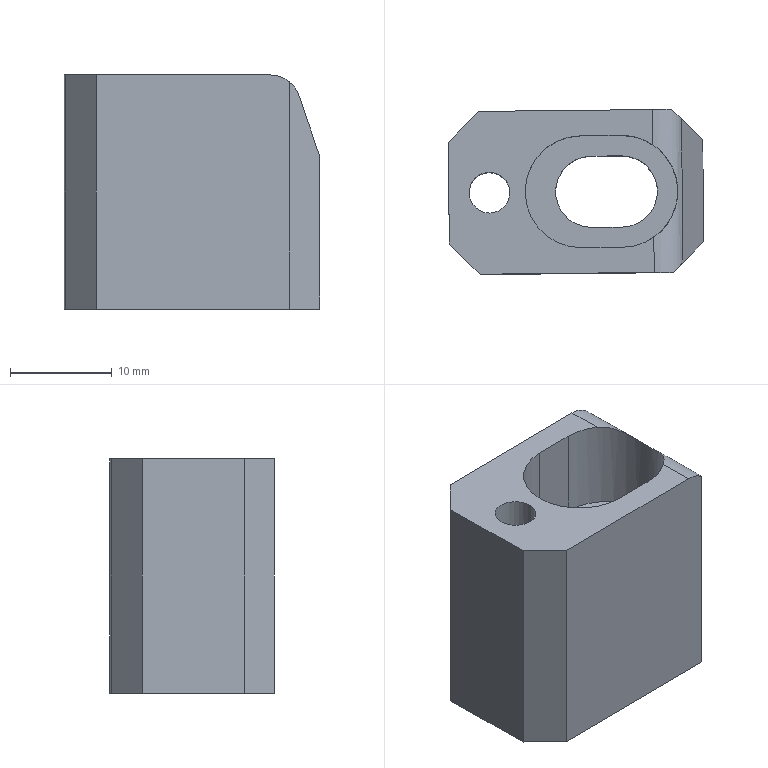Part | NX | features solid 2 | 1 solid | 22 faces | box 25.103 x 16.198 x 23 mm | volume 6273 mm3 | plane 16 | cylinder 6 | commonest cylinder face diameters 7 x2 11 x2 4.001 x1 6 x1
STEP:
#1=CARTESIAN_POINT('',(1618.85,-304.866,17.4));
#2=VERTEX_POINT('',#1);
#3=CARTESIAN_POINT('',(1635.95,-304.687,17.4));
#4=VERTEX_POINT('',#3);
#5=CARTESIAN_POINT('',(1630.849,-304.74,17.4));
#6=DIRECTION('',(0.9999,0.01047,0.));
#7=VECTOR('',#6,1000.);
#8=LINE('',#5,#7);
#9=EDGE_CURVE('',#2,#4,#8,.T.);
#10=ORIENTED_EDGE('',*,*,#9,.F.);
#11=CARTESIAN_POINT('',(1615.881,-307.897,17.4));
#12=VERTEX_POINT('',#11);
#13=CARTESIAN_POINT('',(1620.334,-303.35,17.4));
#14=DIRECTION('',(-0.6997,-0.7145,0.));
#15=VECTOR('',#14,1000.);
#16=LINE('',#13,#15);
#17=EDGE_CURVE('',#2,#12,#16,.T.);
#18=ORIENTED_EDGE('',*,*,#17,.T.);
#19=CARTESIAN_POINT('',(1615.986,-317.896,17.4));
#20=VERTEX_POINT('',#19);
#21=CARTESIAN_POINT('',(1615.934,-312.897,17.4));
#22=DIRECTION('',(-0.01047,0.9999,0.));
#23=VECTOR('',#22,1000.);
#24=LINE('',#21,#23);
#25=EDGE_CURVE('',#20,#12,#24,.T.);
#26=ORIENTED_EDGE('',*,*,#25,.F.);
#27=CARTESIAN_POINT('',(1619.017,-320.865,17.4));
#28=VERTEX_POINT('',#27);
#29=CARTESIAN_POINT('',(1620.533,-322.349,17.4));
#30=DIRECTION('',(0.7145,-0.6997,0.));
#31=VECTOR('',#30,1000.);
#32=LINE('',#29,#31);
#33=EDGE_CURVE('',#20,#28,#32,.T.);
#34=ORIENTED_EDGE('',*,*,#33,.T.);
#35=CARTESIAN_POINT('',(1636.118,-320.686,17.4));
#36=VERTEX_POINT('',#35);
#37=CARTESIAN_POINT('',(1631.017,-320.739,17.4));
#38=DIRECTION('',(-0.9999,-0.01047,0.));
#39=VECTOR('',#38,1000.);
#40=LINE('',#37,#39);
#41=EDGE_CURVE('',#36,#28,#40,.T.);
#42=ORIENTED_EDGE('',*,*,#41,.F.);
#43=CARTESIAN_POINT('',(1636.081,-317.228,17.4));
#44=VERTEX_POINT('',#43);
#45=CARTESIAN_POINT('',(1636.034,-312.686,17.4));
#46=DIRECTION('',(-0.01047,0.9999,0.));
#47=VECTOR('',#46,1000.);
#48=LINE('',#45,#47);
#49=EDGE_CURVE('',#36,#44,#48,.T.);
#50=ORIENTED_EDGE('',*,*,#49,.T.);
#51=CARTESIAN_POINT('',(1632.99,-318.218,17.4));
#52=VERTEX_POINT('',#51);
#53=CARTESIAN_POINT('',(1632.933,-312.719,17.4));
#54=DIRECTION('',(0.,0.,-1.));
#55=DIRECTION('',(-0.1736,0.9848,0.));
#56=AXIS2_PLACEMENT_3D('',#53,#54,#55);
#57=CIRCLE('',#56,5.5);
#58=EDGE_CURVE('',#44,#52,#57,.T.);
#59=ORIENTED_EDGE('',*,*,#58,.T.);
#60=CARTESIAN_POINT('',(1628.99,-318.26,17.4));
#61=VERTEX_POINT('',#60);
#62=CARTESIAN_POINT('',(1630.99,-318.239,17.4));
#63=DIRECTION('',(-0.9999,-0.01047,0.));
#64=VECTOR('',#63,1000.);
#65=LINE('',#62,#64);
#66=EDGE_CURVE('',#52,#61,#65,.T.);
#67=ORIENTED_EDGE('',*,*,#66,.T.);
#68=CARTESIAN_POINT('',(1628.875,-307.261,17.4));
#69=VERTEX_POINT('',#68);
#70=CARTESIAN_POINT('',(1628.933,-312.761,17.4));
#71=DIRECTION('',(0.,0.,-1.));
#72=DIRECTION('',(-0.1736,0.9848,0.));
#73=AXIS2_PLACEMENT_3D('',#70,#71,#72);
#74=CIRCLE('',#73,5.5);
#75=EDGE_CURVE('',#61,#69,#74,.T.);
#76=ORIENTED_EDGE('',*,*,#75,.T.);
#77=CARTESIAN_POINT('',(1632.875,-307.219,17.4));
#78=VERTEX_POINT('',#77);
#79=CARTESIAN_POINT('',(1630.875,-307.24,17.4));
#80=DIRECTION('',(0.9999,0.01047,0.));
#81=VECTOR('',#80,1000.);
#82=LINE('',#79,#81);
#83=EDGE_CURVE('',#69,#78,#82,.T.);
#84=ORIENTED_EDGE('',*,*,#83,.T.);
#85=CARTESIAN_POINT('',(1635.986,-308.144,17.4));
#86=VERTEX_POINT('',#85);
#87=CARTESIAN_POINT('',(1632.933,-312.719,17.4));
#88=DIRECTION('',(0.,0.,-1.));
#89=DIRECTION('',(-0.1736,0.9848,0.));
#90=AXIS2_PLACEMENT_3D('',#87,#88,#89);
#91=CIRCLE('',#90,5.5);
#92=EDGE_CURVE('',#78,#86,#91,.T.);
#93=ORIENTED_EDGE('',*,*,#92,.T.);
#94=CARTESIAN_POINT('',(1636.034,-312.686,17.4));
#95=DIRECTION('',(-0.01047,0.9999,0.));
#96=VECTOR('',#95,1000.);
#97=LINE('',#94,#96);
#98=EDGE_CURVE('',#86,#4,#97,.T.);
#99=ORIENTED_EDGE('',*,*,#98,.T.);
#100=EDGE_LOOP('',(#10,#18,#26,#34,#42,#50,#59,#67,#76,#84,#93,#99));
#101=FACE_BOUND('',#100,.T.);
#102=CARTESIAN_POINT('',(1619.49,-314.806,17.4));
#103=VERTEX_POINT('',#102);
#104=CARTESIAN_POINT('',(1619.933,-312.855,17.4));
#105=DIRECTION('',(0.,0.,-1.));
#106=DIRECTION('',(-0.2215,-0.9751,0.));
#107=AXIS2_PLACEMENT_3D('',#104,#105,#106);
#108=CIRCLE('',#107,2.001);
#109=EDGE_CURVE('',#103,#103,#108,.T.);
#110=ORIENTED_EDGE('',*,*,#109,.T.);
#111=EDGE_LOOP('',(#110));
#112=FACE_BOUND('',#111,.T.);
#113=CARTESIAN_POINT('',(1630.933,-312.74,17.4));
#114=DIRECTION('',(0.,0.,1.));
#115=DIRECTION('',(0.184,-0.9829,0.));
#116=AXIS2_PLACEMENT_3D('',#113,#114,#115);
#117=PLANE('',#116);
#118=ADVANCED_FACE('',(#101,#112),#117,.T.);
#119=CARTESIAN_POINT('',(1620.417,-314.796,-5.6));
#120=VERTEX_POINT('',#119);
#121=CARTESIAN_POINT('',(1619.933,-312.855,-5.6));
#122=DIRECTION('',(0.,0.,-1.));
#123=DIRECTION('',(0.2419,-0.9703,0.));
#124=AXIS2_PLACEMENT_3D('',#121,#122,#123);
#125=CIRCLE('',#124,2.001);
#126=EDGE_CURVE('',#120,#120,#125,.T.);
#127=ORIENTED_EDGE('',*,*,#126,.F.);
#128=EDGE_LOOP('',(#127));
#129=FACE_BOUND('',#128,.T.);
#130=CARTESIAN_POINT('',(1637.849,-304.667,-5.6));
#131=VERTEX_POINT('',#130);
#132=CARTESIAN_POINT('',(1618.85,-304.866,-5.6));
#133=VERTEX_POINT('',#132);
#134=CARTESIAN_POINT('',(1630.849,-304.74,-5.6));
#135=DIRECTION('',(-0.9999,-0.01047,0.));
#136=VECTOR('',#135,1000.);
#137=LINE('',#134,#136);
#138=EDGE_CURVE('',#131,#133,#137,.T.);
#139=ORIENTED_EDGE('',*,*,#138,.F.);
#140=CARTESIAN_POINT('',(1640.88,-307.635,-5.6));
#141=VERTEX_POINT('',#140);
#142=CARTESIAN_POINT('',(1638.354,-305.161,-5.6));
#143=DIRECTION('',(0.7145,-0.6997,0.));
#144=VECTOR('',#143,1000.);
#145=LINE('',#142,#144);
#146=EDGE_CURVE('',#131,#141,#145,.T.);
#147=ORIENTED_EDGE('',*,*,#146,.T.);
#148=CARTESIAN_POINT('',(1640.985,-317.635,-5.6));
#149=VERTEX_POINT('',#148);
#150=CARTESIAN_POINT('',(1640.932,-312.635,-5.6));
#151=DIRECTION('',(-0.01047,0.9999,0.));
#152=VECTOR('',#151,1000.);
#153=LINE('',#150,#152);
#154=EDGE_CURVE('',#149,#141,#153,.T.);
#155=ORIENTED_EDGE('',*,*,#154,.F.);
#156=CARTESIAN_POINT('',(1638.016,-320.666,-5.6));
#157=VERTEX_POINT('',#156);
#158=CARTESIAN_POINT('',(1638.511,-320.161,-5.6));
#159=DIRECTION('',(-0.6997,-0.7145,0.));
#160=VECTOR('',#159,1000.);
#161=LINE('',#158,#160);
#162=EDGE_CURVE('',#149,#157,#161,.T.);
#163=ORIENTED_EDGE('',*,*,#162,.T.);
#164=CARTESIAN_POINT('',(1619.017,-320.865,-5.6));
#165=VERTEX_POINT('',#164);
#166=CARTESIAN_POINT('',(1631.017,-320.739,-5.6));
#167=DIRECTION('',(0.9999,0.01047,0.));
#168=VECTOR('',#167,1000.);
#169=LINE('',#166,#168);
#170=EDGE_CURVE('',#165,#157,#169,.T.);
#171=ORIENTED_EDGE('',*,*,#170,.F.);
#172=CARTESIAN_POINT('',(1615.986,-317.896,-5.6));
#173=VERTEX_POINT('',#172);
#174=CARTESIAN_POINT('',(1620.028,-321.854,-5.6));
#175=DIRECTION('',(-0.7145,0.6997,0.));
#176=VECTOR('',#175,1000.);
#177=LINE('',#174,#176);
#178=EDGE_CURVE('',#165,#173,#177,.T.);
#179=ORIENTED_EDGE('',*,*,#178,.T.);
#180=CARTESIAN_POINT('',(1615.881,-307.897,-5.6));
#181=VERTEX_POINT('',#180);
#182=CARTESIAN_POINT('',(1615.934,-312.897,-5.6));
#183=DIRECTION('',(0.01047,-0.9999,0.));
#184=VECTOR('',#183,1000.);
#185=LINE('',#182,#184);
#186=EDGE_CURVE('',#181,#173,#185,.T.);
#187=ORIENTED_EDGE('',*,*,#186,.F.);
#188=CARTESIAN_POINT('',(1619.839,-303.855,-5.6));
#189=DIRECTION('',(0.6997,0.7145,0.));
#190=VECTOR('',#189,1000.);
#191=LINE('',#188,#190);
#192=EDGE_CURVE('',#181,#133,#191,.T.);
#193=ORIENTED_EDGE('',*,*,#192,.T.);
#194=EDGE_LOOP('',(#139,#147,#155,#163,#171,#179,#187,#193));
#195=FACE_BOUND('',#194,.T.);
#196=CARTESIAN_POINT('',(1632.969,-316.218,-5.6));
#197=VERTEX_POINT('',#196);
#198=CARTESIAN_POINT('',(1632.896,-309.219,-5.6));
#199=VERTEX_POINT('',#198);
#200=CARTESIAN_POINT('',(1632.933,-312.719,-5.6));
#201=DIRECTION('',(0.,0.,1.));
#202=DIRECTION('',(0.2419,-0.9703,0.));
#203=AXIS2_PLACEMENT_3D('',#200,#201,#202);
#204=CIRCLE('',#203,3.5);
#205=EDGE_CURVE('',#197,#199,#204,.T.);
#206=ORIENTED_EDGE('',*,*,#205,.T.);
#207=CARTESIAN_POINT('',(1629.896,-309.25,-5.6));
#208=VERTEX_POINT('',#207);
#209=CARTESIAN_POINT('',(1630.896,-309.24,-5.6));
#210=DIRECTION('',(-0.9999,-0.01047,0.));
#211=VECTOR('',#210,1000.);
#212=LINE('',#209,#211);
#213=EDGE_CURVE('',#199,#208,#212,.T.);
#214=ORIENTED_EDGE('',*,*,#213,.T.);
#215=CARTESIAN_POINT('',(1629.969,-316.25,-5.6));
#216=VERTEX_POINT('',#215);
#217=CARTESIAN_POINT('',(1629.933,-312.75,-5.6));
#218=DIRECTION('',(0.,0.,1.));
#219=DIRECTION('',(0.2419,-0.9703,0.));
#220=AXIS2_PLACEMENT_3D('',#217,#218,#219);
#221=CIRCLE('',#220,3.5);
#222=EDGE_CURVE('',#208,#216,#221,.T.);
#223=ORIENTED_EDGE('',*,*,#222,.T.);
#224=CARTESIAN_POINT('',(1630.969,-316.239,-5.6));
#225=DIRECTION('',(0.9999,0.01047,0.));
#226=VECTOR('',#225,1000.);
#227=LINE('',#224,#226);
#228=EDGE_CURVE('',#216,#197,#227,.T.);
#229=ORIENTED_EDGE('',*,*,#228,.T.);
#230=EDGE_LOOP('',(#206,#214,#223,#229));
#231=FACE_BOUND('',#230,.T.);
#232=CARTESIAN_POINT('',(1630.933,-312.74,-5.6));
#233=DIRECTION('',(0.,0.,-1.));
#234=DIRECTION('',(-0.184,0.9829,0.));
#235=AXIS2_PLACEMENT_3D('',#232,#233,#234);
#236=PLANE('',#235);
#237=ADVANCED_FACE('',(#129,#195,#231),#236,.T.);
#238=ORIENTED_EDGE('',*,*,#154,.T.);
#239=CARTESIAN_POINT('',(1640.88,-307.635,9.4));
#240=VERTEX_POINT('',#239);
#241=CARTESIAN_POINT('',(1640.88,-307.635,2.4));
#242=DIRECTION('',(0.,0.,1.));
#243=VECTOR('',#242,1000.);
#244=LINE('',#241,#243);
#245=EDGE_CURVE('',#141,#240,#244,.T.);
#246=ORIENTED_EDGE('',*,*,#245,.T.);
#247=CARTESIAN_POINT('',(1640.985,-317.635,9.4));
#248=VERTEX_POINT('',#247);
#249=CARTESIAN_POINT('',(1640.932,-312.635,9.4));
#250=DIRECTION('',(0.01047,-0.9999,0.));
#251=VECTOR('',#250,1000.);
#252=LINE('',#249,#251);
#253=EDGE_CURVE('',#240,#248,#252,.T.);
#254=ORIENTED_EDGE('',*,*,#253,.T.);
#255=CARTESIAN_POINT('',(1640.985,-317.635,2.4));
#256=DIRECTION('',(0.,0.,-1.));
#257=VECTOR('',#256,1000.);
#258=LINE('',#255,#257);
#259=EDGE_CURVE('',#248,#149,#258,.T.);
#260=ORIENTED_EDGE('',*,*,#259,.T.);
#261=EDGE_LOOP('',(#238,#246,#254,#260));
#262=FACE_BOUND('',#261,.T.);
#263=CARTESIAN_POINT('',(1640.932,-312.635,2.4));
#264=DIRECTION('',(0.9999,0.01047,0.));
#265=DIRECTION('',(0.01047,-0.9999,0.));
#266=AXIS2_PLACEMENT_3D('',#263,#264,#265);
#267=PLANE('',#266);
#268=ADVANCED_FACE('',(#262),#267,.T.);
#269=ORIENTED_EDGE('',*,*,#170,.T.);
#270=CARTESIAN_POINT('',(1638.016,-320.666,16.723));
#271=VERTEX_POINT('',#270);
#272=CARTESIAN_POINT('',(1638.016,-320.666,2.4));
#273=DIRECTION('',(0.,0.,1.));
#274=VECTOR('',#273,1000.);
#275=LINE('',#272,#274);
#276=EDGE_CURVE('',#157,#271,#275,.T.);
#277=ORIENTED_EDGE('',*,*,#276,.T.);
#278=CARTESIAN_POINT('',(1636.118,-320.686,14.4));
#279=DIRECTION('',(0.01047,-0.9999,0.));
#280=DIRECTION('',(0.9999,0.01047,0.));
#281=AXIS2_PLACEMENT_3D('',#278,#279,#280);
#282=CIRCLE('',#281,3.);
#283=EDGE_CURVE('',#271,#36,#282,.T.);
#284=ORIENTED_EDGE('',*,*,#283,.T.);
#285=ORIENTED_EDGE('',*,*,#41,.T.);
#286=CARTESIAN_POINT('',(1619.017,-320.865,2.4));
#287=DIRECTION('',(0.,0.,-1.));
#288=VECTOR('',#287,1000.);
#289=LINE('',#286,#288);
#290=EDGE_CURVE('',#28,#165,#289,.T.);
#291=ORIENTED_EDGE('',*,*,#290,.T.);
#292=EDGE_LOOP('',(#269,#277,#284,#285,#291));
#293=FACE_BOUND('',#292,.T.);
#294=CARTESIAN_POINT('',(1631.017,-320.739,2.4));
#295=DIRECTION('',(0.01047,-0.9999,0.));
#296=DIRECTION('',(-0.9999,-0.01047,0.));
#297=AXIS2_PLACEMENT_3D('',#294,#295,#296);
#298=PLANE('',#297);
#299=ADVANCED_FACE('',(#293),#298,.T.);
#300=ORIENTED_EDGE('',*,*,#25,.T.);
#301=CARTESIAN_POINT('',(1615.881,-307.897,2.4));
#302=DIRECTION('',(0.,0.,-1.));
#303=VECTOR('',#302,1000.);
#304=LINE('',#301,#303);
#305=EDGE_CURVE('',#12,#181,#304,.T.);
#306=ORIENTED_EDGE('',*,*,#305,.T.);
#307=ORIENTED_EDGE('',*,*,#186,.T.);
#308=CARTESIAN_POINT('',(1615.986,-317.896,2.4));
#309=DIRECTION('',(0.,0.,1.));
#310=VECTOR('',#309,1000.);
#311=LINE('',#308,#310);
#312=EDGE_CURVE('',#173,#20,#311,.T.);
#313=ORIENTED_EDGE('',*,*,#312,.T.);
#314=EDGE_LOOP('',(#300,#306,#307,#313));
#315=FACE_BOUND('',#314,.T.);
#316=CARTESIAN_POINT('',(1615.934,-312.897,2.4));
#317=DIRECTION('',(-0.9999,-0.01047,0.));
#318=DIRECTION('',(-0.01047,0.9999,0.));
#319=AXIS2_PLACEMENT_3D('',#316,#317,#318);
#320=PLANE('',#319);
#321=ADVANCED_FACE('',(#315),#320,.T.);
#322=CARTESIAN_POINT('',(1637.849,-304.667,16.723));
#323=VERTEX_POINT('',#322);
#324=CARTESIAN_POINT('',(1635.95,-304.687,14.4));
#325=DIRECTION('',(-0.01047,0.9999,0.));
#326=DIRECTION('',(-0.9999,-0.01047,0.));
#327=AXIS2_PLACEMENT_3D('',#324,#325,#326);
#328=CIRCLE('',#327,3.);
#329=EDGE_CURVE('',#4,#323,#328,.T.);
#330=ORIENTED_EDGE('',*,*,#329,.T.);
#331=CARTESIAN_POINT('',(1637.849,-304.667,2.4));
#332=DIRECTION('',(0.,0.,-1.));
#333=VECTOR('',#332,1000.);
#334=LINE('',#331,#333);
#335=EDGE_CURVE('',#323,#131,#334,.T.);
#336=ORIENTED_EDGE('',*,*,#335,.T.);
#337=ORIENTED_EDGE('',*,*,#138,.T.);
#338=CARTESIAN_POINT('',(1618.85,-304.866,2.4));
#339=DIRECTION('',(0.,0.,1.));
#340=VECTOR('',#339,1000.);
#341=LINE('',#338,#340);
#342=EDGE_CURVE('',#133,#2,#341,.T.);
#343=ORIENTED_EDGE('',*,*,#342,.T.);
#344=ORIENTED_EDGE('',*,*,#9,.T.);
#345=EDGE_LOOP('',(#330,#336,#337,#343,#344));
#346=FACE_BOUND('',#345,.T.);
#347=CARTESIAN_POINT('',(1630.849,-304.74,2.4));
#348=DIRECTION('',(-0.01047,0.9999,0.));
#349=DIRECTION('',(0.9999,0.01047,0.));
#350=AXIS2_PLACEMENT_3D('',#347,#348,#349);
#351=PLANE('',#350);
#352=ADVANCED_FACE('',(#346),#351,.T.);
#353=CARTESIAN_POINT('',(1629.896,-309.25,8.4));
#354=VERTEX_POINT('',#353);
#355=CARTESIAN_POINT('',(1629.969,-316.25,8.4));
#356=VERTEX_POINT('',#355);
#357=CARTESIAN_POINT('',(1629.933,-312.75,8.4));
#358=DIRECTION('',(0.,0.,1.));
#359=DIRECTION('',(0.1736,-0.9848,0.));
#360=AXIS2_PLACEMENT_3D('',#357,#358,#359);
#361=CIRCLE('',#360,3.5);
#362=EDGE_CURVE('',#354,#356,#361,.T.);
#363=ORIENTED_EDGE('',*,*,#362,.F.);
#364=CARTESIAN_POINT('',(1632.896,-309.219,8.4));
#365=VERTEX_POINT('',#364);
#366=CARTESIAN_POINT('',(1629.995,-309.249,8.4));
#367=DIRECTION('',(0.9999,0.01047,0.));
#368=VECTOR('',#367,1000.);
#369=LINE('',#366,#368);
#370=EDGE_CURVE('',#354,#365,#369,.T.);
#371=ORIENTED_EDGE('',*,*,#370,.T.);
#372=CARTESIAN_POINT('',(1632.969,-316.218,8.4));
#373=VERTEX_POINT('',#372);
#374=CARTESIAN_POINT('',(1632.933,-312.719,8.4));
#375=DIRECTION('',(0.,0.,-1.));
#376=DIRECTION('',(0.1736,-0.9848,0.));
#377=AXIS2_PLACEMENT_3D('',#374,#375,#376);
#378=CIRCLE('',#377,3.5);
#379=EDGE_CURVE('',#365,#373,#378,.T.);
#380=ORIENTED_EDGE('',*,*,#379,.T.);
#381=CARTESIAN_POINT('',(1630.068,-316.249,8.4));
#382=DIRECTION('',(-0.9999,-0.01047,0.));
#383=VECTOR('',#382,1000.);
#384=LINE('',#381,#383);
#385=EDGE_CURVE('',#373,#356,#384,.T.);
#386=ORIENTED_EDGE('',*,*,#385,.T.);
#387=EDGE_LOOP('',(#363,#371,#380,#386));
#388=FACE_BOUND('',#387,.T.);
#389=CARTESIAN_POINT('',(1632.875,-307.219,8.4));
#390=VERTEX_POINT('',#389);
#391=CARTESIAN_POINT('',(1632.99,-318.218,8.4));
#392=VERTEX_POINT('',#391);
#393=CARTESIAN_POINT('',(1632.933,-312.719,8.4));
#394=DIRECTION('',(0.,0.,-1.));
#395=DIRECTION('',(0.1736,-0.9848,0.));
#396=AXIS2_PLACEMENT_3D('',#393,#394,#395);
#397=CIRCLE('',#396,5.5);
#398=EDGE_CURVE('',#390,#392,#397,.T.);
#399=ORIENTED_EDGE('',*,*,#398,.F.);
#400=CARTESIAN_POINT('',(1628.875,-307.261,8.4));
#401=VERTEX_POINT('',#400);
#402=CARTESIAN_POINT('',(1628.875,-307.261,8.4));
#403=DIRECTION('',(-0.9999,-0.01047,0.));
#404=VECTOR('',#403,1000.);
#405=LINE('',#402,#404);
#406=EDGE_CURVE('',#390,#401,#405,.T.);
#407=ORIENTED_EDGE('',*,*,#406,.T.);
#408=CARTESIAN_POINT('',(1628.99,-318.26,8.4));
#409=VERTEX_POINT('',#408);
#410=CARTESIAN_POINT('',(1628.933,-312.761,8.4));
#411=DIRECTION('',(0.,0.,1.));
#412=DIRECTION('',(0.1736,-0.9848,0.));
#413=AXIS2_PLACEMENT_3D('',#410,#411,#412);
#414=CIRCLE('',#413,5.5);
#415=EDGE_CURVE('',#401,#409,#414,.T.);
#416=ORIENTED_EDGE('',*,*,#415,.T.);
#417=CARTESIAN_POINT('',(1628.99,-318.26,8.4));
#418=DIRECTION('',(0.9999,0.01047,0.));
#419=VECTOR('',#418,1000.);
#420=LINE('',#417,#419);
#421=EDGE_CURVE('',#409,#392,#420,.T.);
#422=ORIENTED_EDGE('',*,*,#421,.T.);
#423=EDGE_LOOP('',(#399,#407,#416,#422));
#424=FACE_BOUND('',#423,.T.);
#425=CARTESIAN_POINT('',(1628.933,-312.761,8.4));
#426=DIRECTION('',(0.,0.,-1.));
#427=DIRECTION('',(-0.1736,0.9848,0.));
#428=AXIS2_PLACEMENT_3D('',#425,#426,#427);
#429=PLANE('',#428);
#430=ADVANCED_FACE('',(#388,#424),#429,.F.);
#431=ORIENTED_EDGE('',*,*,#222,.F.);
#432=CARTESIAN_POINT('',(1629.896,-309.25,5.4));
#433=DIRECTION('',(0.,0.,1.));
#434=VECTOR('',#433,1000.);
#435=LINE('',#432,#434);
#436=EDGE_CURVE('',#208,#354,#435,.T.);
#437=ORIENTED_EDGE('',*,*,#436,.T.);
#438=ORIENTED_EDGE('',*,*,#362,.T.);
#439=CARTESIAN_POINT('',(1629.969,-316.25,5.4));
#440=DIRECTION('',(0.,0.,-1.));
#441=VECTOR('',#440,1000.);
#442=LINE('',#439,#441);
#443=EDGE_CURVE('',#356,#216,#442,.T.);
#444=ORIENTED_EDGE('',*,*,#443,.T.);
#445=EDGE_LOOP('',(#431,#437,#438,#444));
#446=FACE_BOUND('',#445,.T.);
#447=CARTESIAN_POINT('',(1629.933,-312.75,22.4));
#448=DIRECTION('',(0.,0.,-1.));
#449=DIRECTION('',(0.1736,-0.9848,0.));
#450=AXIS2_PLACEMENT_3D('',#447,#448,#449);
#451=CYLINDRICAL_SURFACE('',#450,3.5);
#452=ADVANCED_FACE('',(#446),#451,.F.);
#453=ORIENTED_EDGE('',*,*,#415,.F.);
#454=CARTESIAN_POINT('',(1628.875,-307.261,12.9));
#455=DIRECTION('',(0.,0.,1.));
#456=VECTOR('',#455,1000.);
#457=LINE('',#454,#456);
#458=EDGE_CURVE('',#401,#69,#457,.T.);
#459=ORIENTED_EDGE('',*,*,#458,.T.);
#460=ORIENTED_EDGE('',*,*,#75,.F.);
#461=CARTESIAN_POINT('',(1628.99,-318.26,12.9));
#462=DIRECTION('',(0.,0.,-1.));
#463=VECTOR('',#462,1000.);
#464=LINE('',#461,#463);
#465=EDGE_CURVE('',#61,#409,#464,.T.);
#466=ORIENTED_EDGE('',*,*,#465,.T.);
#467=EDGE_LOOP('',(#453,#459,#460,#466));
#468=FACE_BOUND('',#467,.T.);
#469=CARTESIAN_POINT('',(1628.933,-312.761,22.4));
#470=DIRECTION('',(0.,0.,-1.));
#471=DIRECTION('',(0.1736,-0.9848,0.));
#472=AXIS2_PLACEMENT_3D('',#469,#470,#471);
#473=CYLINDRICAL_SURFACE('',#472,5.5);
#474=ADVANCED_FACE('',(#468),#473,.F.);
#475=ORIENTED_EDGE('',*,*,#379,.F.);
#476=CARTESIAN_POINT('',(1632.896,-309.219,5.4));
#477=DIRECTION('',(0.,0.,-1.));
#478=VECTOR('',#477,1000.);
#479=LINE('',#476,#478);
#480=EDGE_CURVE('',#365,#199,#479,.T.);
#481=ORIENTED_EDGE('',*,*,#480,.T.);
#482=ORIENTED_EDGE('',*,*,#205,.F.);
#483=CARTESIAN_POINT('',(1632.969,-316.218,5.4));
#484=DIRECTION('',(0.,0.,1.));
#485=VECTOR('',#484,1000.);
#486=LINE('',#483,#485);
#487=EDGE_CURVE('',#197,#373,#486,.T.);
#488=ORIENTED_EDGE('',*,*,#487,.T.);
#489=EDGE_LOOP('',(#475,#481,#482,#488));
#490=FACE_BOUND('',#489,.T.);
#491=CARTESIAN_POINT('',(1632.933,-312.719,22.4));
#492=DIRECTION('',(0.,0.,-1.));
#493=DIRECTION('',(0.1736,-0.9848,0.));
#494=AXIS2_PLACEMENT_3D('',#491,#492,#493);
#495=CYLINDRICAL_SURFACE('',#494,3.5);
#496=ADVANCED_FACE('',(#490),#495,.F.);
#497=ORIENTED_EDGE('',*,*,#92,.F.);
#498=CARTESIAN_POINT('',(1632.875,-307.219,12.9));
#499=DIRECTION('',(0.,0.,-1.));
#500=VECTOR('',#499,1000.);
#501=LINE('',#498,#500);
#502=EDGE_CURVE('',#78,#390,#501,.T.);
#503=ORIENTED_EDGE('',*,*,#502,.T.);
#504=ORIENTED_EDGE('',*,*,#398,.T.);
#505=CARTESIAN_POINT('',(1632.99,-318.218,12.9));
#506=DIRECTION('',(0.,0.,1.));
#507=VECTOR('',#506,1000.);
#508=LINE('',#505,#507);
#509=EDGE_CURVE('',#392,#52,#508,.T.);
#510=ORIENTED_EDGE('',*,*,#509,.T.);
#511=ORIENTED_EDGE('',*,*,#58,.F.);
#512=CARTESIAN_POINT('',(1636.081,-317.228,17.4));
#513=CARTESIAN_POINT('',(1636.844,-316.696,17.4));
#514=CARTESIAN_POINT('',(1638.006,-315.341,16.852));
#515=CARTESIAN_POINT('',(1638.659,-312.657,15.876));
#516=CARTESIAN_POINT('',(1637.95,-309.991,16.852));
#517=CARTESIAN_POINT('',(1636.759,-308.66,17.4));
#518=CARTESIAN_POINT('',(1635.986,-308.144,17.4));
#519=B_SPLINE_CURVE_WITH_KNOTS('',3,(#512,#513,#514,#515,#516,#517,#518),.UNSPECIFIED.,.F.,.F.,(4,1,1,1,4),(0.,0.002735,0.00547,0.008205,0.01094),.UNSPECIFIED.);
#520=EDGE_CURVE('',#44,#86,#519,.T.);
#521=ORIENTED_EDGE('',*,*,#520,.T.);
#522=EDGE_LOOP('',(#497,#503,#504,#510,#511,#521));
#523=FACE_BOUND('',#522,.T.);
#524=CARTESIAN_POINT('',(1632.933,-312.719,22.4));
#525=DIRECTION('',(0.,0.,-1.));
#526=DIRECTION('',(0.1736,-0.9848,0.));
#527=AXIS2_PLACEMENT_3D('',#524,#525,#526);
#528=CYLINDRICAL_SURFACE('',#527,5.5);
#529=ADVANCED_FACE('',(#523),#528,.F.);
#530=ORIENTED_EDGE('',*,*,#253,.F.);
#531=CARTESIAN_POINT('',(1638.796,-305.594,15.378));
#532=VERTEX_POINT('',#531);
#533=CARTESIAN_POINT('',(1641.366,-308.111,8.007));
#534=DIRECTION('',(-0.3133,0.3068,0.8987));
#535=VECTOR('',#534,1000.);
#536=LINE('',#533,#535);
#537=EDGE_CURVE('',#240,#532,#536,.T.);
#538=ORIENTED_EDGE('',*,*,#537,.T.);
#539=CARTESIAN_POINT('',(1638.943,-319.719,15.378));
#540=VERTEX_POINT('',#539);
#541=CARTESIAN_POINT('',(1638.87,-312.656,15.378));
#542=DIRECTION('',(0.01047,-0.9999,0.));
#543=VECTOR('',#542,1000.);
#544=LINE('',#541,#543);
#545=EDGE_CURVE('',#532,#540,#544,.T.);
#546=ORIENTED_EDGE('',*,*,#545,.T.);
#547=CARTESIAN_POINT('',(1641.46,-317.149,8.007));
#548=DIRECTION('',(0.3068,0.3133,-0.8987));
#549=VECTOR('',#548,1000.);
#550=LINE('',#547,#549);
#551=EDGE_CURVE('',#540,#248,#550,.T.);
#552=ORIENTED_EDGE('',*,*,#551,.T.);
#553=EDGE_LOOP('',(#530,#538,#546,#552));
#554=FACE_BOUND('',#553,.T.);
#555=CARTESIAN_POINT('',(1640.932,-312.635,9.4));
#556=DIRECTION('',(-0.9453,-0.009899,-0.3262));
#557=DIRECTION('',(-0.01047,0.9999,0.));
#558=AXIS2_PLACEMENT_3D('',#555,#556,#557);
#559=PLANE('',#558);
#560=ADVANCED_FACE('',(#554),#559,.F.);
#561=ORIENTED_EDGE('',*,*,#545,.F.);
#562=CARTESIAN_POINT('',(1635.93,-302.788,14.4));
#563=DIRECTION('',(-0.6997,-0.7145,0.));
#564=DIRECTION('',(0.7145,-0.6997,0.));
#565=AXIS2_PLACEMENT_3D('',#562,#563,#564);
#566=ELLIPSE('',#565,4.243,3.);
#567=EDGE_CURVE('',#532,#323,#566,.T.);
#568=ORIENTED_EDGE('',*,*,#567,.T.);
#569=ORIENTED_EDGE('',*,*,#329,.F.);
#570=ORIENTED_EDGE('',*,*,#98,.F.);
#571=ORIENTED_EDGE('',*,*,#520,.F.);
#572=ORIENTED_EDGE('',*,*,#49,.F.);
#573=ORIENTED_EDGE('',*,*,#283,.F.);
#574=CARTESIAN_POINT('',(1636.137,-322.584,14.4));
#575=DIRECTION('',(-0.7145,0.6997,0.));
#576=DIRECTION('',(-0.6997,-0.7145,0.));
#577=AXIS2_PLACEMENT_3D('',#574,#575,#576);
#578=ELLIPSE('',#577,4.243,3.);
#579=EDGE_CURVE('',#271,#540,#578,.T.);
#580=ORIENTED_EDGE('',*,*,#579,.T.);
#581=EDGE_LOOP('',(#561,#568,#569,#570,#571,#572,#573,#580));
#582=FACE_BOUND('',#581,.T.);
#583=CARTESIAN_POINT('',(1636.034,-312.686,14.4));
#584=DIRECTION('',(0.01047,-0.9999,0.));
#585=DIRECTION('',(-0.9999,-0.01047,0.));
#586=AXIS2_PLACEMENT_3D('',#583,#584,#585);
#587=CYLINDRICAL_SURFACE('',#586,3.);
#588=ADVANCED_FACE('',(#582),#587,.T.);
#589=ORIENTED_EDGE('',*,*,#66,.F.);
#590=ORIENTED_EDGE('',*,*,#509,.F.);
#591=ORIENTED_EDGE('',*,*,#421,.F.);
#592=ORIENTED_EDGE('',*,*,#465,.F.);
#593=EDGE_LOOP('',(#589,#590,#591,#592));
#594=FACE_BOUND('',#593,.T.);
#595=CARTESIAN_POINT('',(1630.026,-318.249,22.4));
#596=DIRECTION('',(0.01047,-0.9999,0.));
#597=DIRECTION('',(0.,0.,1.));
#598=AXIS2_PLACEMENT_3D('',#595,#596,#597);
#599=PLANE('',#598);
#600=ADVANCED_FACE('',(#594),#599,.F.);
#601=ORIENTED_EDGE('',*,*,#385,.F.);
#602=ORIENTED_EDGE('',*,*,#487,.F.);
#603=ORIENTED_EDGE('',*,*,#228,.F.);
#604=ORIENTED_EDGE('',*,*,#443,.F.);
#605=EDGE_LOOP('',(#601,#602,#603,#604));
#606=FACE_BOUND('',#605,.T.);
#607=CARTESIAN_POINT('',(1630.068,-316.249,22.4));
#608=DIRECTION('',(0.01047,-0.9999,0.));
#609=DIRECTION('',(0.,0.,1.));
#610=AXIS2_PLACEMENT_3D('',#607,#608,#609);
#611=PLANE('',#610);
#612=ADVANCED_FACE('',(#606),#611,.F.);
#613=ORIENTED_EDGE('',*,*,#213,.F.);
#614=ORIENTED_EDGE('',*,*,#480,.F.);
#615=ORIENTED_EDGE('',*,*,#370,.F.);
#616=ORIENTED_EDGE('',*,*,#436,.F.);
#617=EDGE_LOOP('',(#613,#614,#615,#616));
#618=FACE_BOUND('',#617,.T.);
#619=CARTESIAN_POINT('',(1629.995,-309.249,22.4));
#620=DIRECTION('',(-0.01047,0.9999,0.));
#621=DIRECTION('',(0.,0.,-1.));
#622=AXIS2_PLACEMENT_3D('',#619,#620,#621);
#623=PLANE('',#622);
#624=ADVANCED_FACE('',(#618),#623,.F.);
#625=ORIENTED_EDGE('',*,*,#406,.F.);
#626=ORIENTED_EDGE('',*,*,#502,.F.);
#627=ORIENTED_EDGE('',*,*,#83,.F.);
#628=ORIENTED_EDGE('',*,*,#458,.F.);
#629=EDGE_LOOP('',(#625,#626,#627,#628));
#630=FACE_BOUND('',#629,.T.);
#631=CARTESIAN_POINT('',(1629.911,-307.25,22.4));
#632=DIRECTION('',(-0.01047,0.9999,0.));
#633=DIRECTION('',(0.,0.,-1.));
#634=AXIS2_PLACEMENT_3D('',#631,#632,#633);
#635=PLANE('',#634);
#636=ADVANCED_FACE('',(#630),#635,.F.);
#637=ORIENTED_EDGE('',*,*,#192,.F.);
#638=ORIENTED_EDGE('',*,*,#305,.F.);
#639=ORIENTED_EDGE('',*,*,#17,.F.);
#640=ORIENTED_EDGE('',*,*,#342,.F.);
#641=EDGE_LOOP('',(#637,#638,#639,#640));
#642=FACE_BOUND('',#641,.T.);
#643=CARTESIAN_POINT('',(1618.85,-304.866,2.4));
#644=DIRECTION('',(0.7145,-0.6997,0.));
#645=DIRECTION('',(0.,0.,-1.));
#646=AXIS2_PLACEMENT_3D('',#643,#644,#645);
#647=PLANE('',#646);
#648=ADVANCED_FACE('',(#642),#647,.F.);
#649=ORIENTED_EDGE('',*,*,#178,.F.);
#650=ORIENTED_EDGE('',*,*,#290,.F.);
#651=ORIENTED_EDGE('',*,*,#33,.F.);
#652=ORIENTED_EDGE('',*,*,#312,.F.);
#653=EDGE_LOOP('',(#649,#650,#651,#652));
#654=FACE_BOUND('',#653,.T.);
#655=CARTESIAN_POINT('',(1615.986,-317.896,2.4));
#656=DIRECTION('',(0.6997,0.7145,0.));
#657=DIRECTION('',(0.,0.,-1.));
#658=AXIS2_PLACEMENT_3D('',#655,#656,#657);
#659=PLANE('',#658);
#660=ADVANCED_FACE('',(#654),#659,.F.);
#661=ORIENTED_EDGE('',*,*,#162,.F.);
#662=ORIENTED_EDGE('',*,*,#259,.F.);
#663=ORIENTED_EDGE('',*,*,#551,.F.);
#664=ORIENTED_EDGE('',*,*,#579,.F.);
#665=ORIENTED_EDGE('',*,*,#276,.F.);
#666=EDGE_LOOP('',(#661,#662,#663,#664,#665));
#667=FACE_BOUND('',#666,.T.);
#668=CARTESIAN_POINT('',(1638.016,-320.666,2.4));
#669=DIRECTION('',(-0.7145,0.6997,0.));
#670=DIRECTION('',(0.,0.,-1.));
#671=AXIS2_PLACEMENT_3D('',#668,#669,#670);
#672=PLANE('',#671);
#673=ADVANCED_FACE('',(#667),#672,.F.);
#674=ORIENTED_EDGE('',*,*,#146,.F.);
#675=ORIENTED_EDGE('',*,*,#335,.F.);
#676=ORIENTED_EDGE('',*,*,#567,.F.);
#677=ORIENTED_EDGE('',*,*,#537,.F.);
#678=ORIENTED_EDGE('',*,*,#245,.F.);
#679=EDGE_LOOP('',(#674,#675,#676,#677,#678));
#680=FACE_BOUND('',#679,.T.);
#681=CARTESIAN_POINT('',(1640.88,-307.635,2.4));
#682=DIRECTION('',(-0.6997,-0.7145,0.));
#683=DIRECTION('',(0.,0.,-1.));
#684=AXIS2_PLACEMENT_3D('',#681,#682,#683);
#685=PLANE('',#684);
#686=ADVANCED_FACE('',(#680),#685,.F.);
#687=ORIENTED_EDGE('',*,*,#109,.F.);
#688=EDGE_LOOP('',(#687));
#689=FACE_BOUND('',#688,.T.);
#690=ORIENTED_EDGE('',*,*,#126,.T.);
#691=EDGE_LOOP('',(#690));
#692=FACE_BOUND('',#691,.T.);
#693=CARTESIAN_POINT('',(1619.933,-312.855,17.4));
#694=DIRECTION('',(0.,0.,-1.));
#695=DIRECTION('',(-0.2215,-0.9751,0.));
#696=AXIS2_PLACEMENT_3D('',#693,#694,#695);
#697=CYLINDRICAL_SURFACE('',#696,2.001);
#698=ADVANCED_FACE('',(#689,#692),#697,.F.);
#699=CLOSED_SHELL('',(#118,#237,#268,#299,#321,#352,#430,#452,#474,#496,#529,#560,#588,#600,#612,#624,#636,#648,#660,#673,#686,#698));
#700=MANIFOLD_SOLID_BREP('',#699);
#701=(LENGTH_UNIT()NAMED_UNIT(*)SI_UNIT(.MILLI.,.METRE.));
#702=UNCERTAINTY_MEASURE_WITH_UNIT(LENGTH_MEASURE(0.0508),#701,'','');
#703=(NAMED_UNIT(*)PLANE_ANGLE_UNIT()SI_UNIT($,.RADIAN.));
#704=(NAMED_UNIT(*)SI_UNIT($,.STERADIAN.)SOLID_ANGLE_UNIT());
#705=(GEOMETRIC_REPRESENTATION_CONTEXT(3)GLOBAL_UNCERTAINTY_ASSIGNED_CONTEXT((#702))GLOBAL_UNIT_ASSIGNED_CONTEXT((#701,#703,#704))REPRESENTATION_CONTEXT('',''));
#706=ADVANCED_BREP_SHAPE_REPRESENTATION('',(#700),#705);